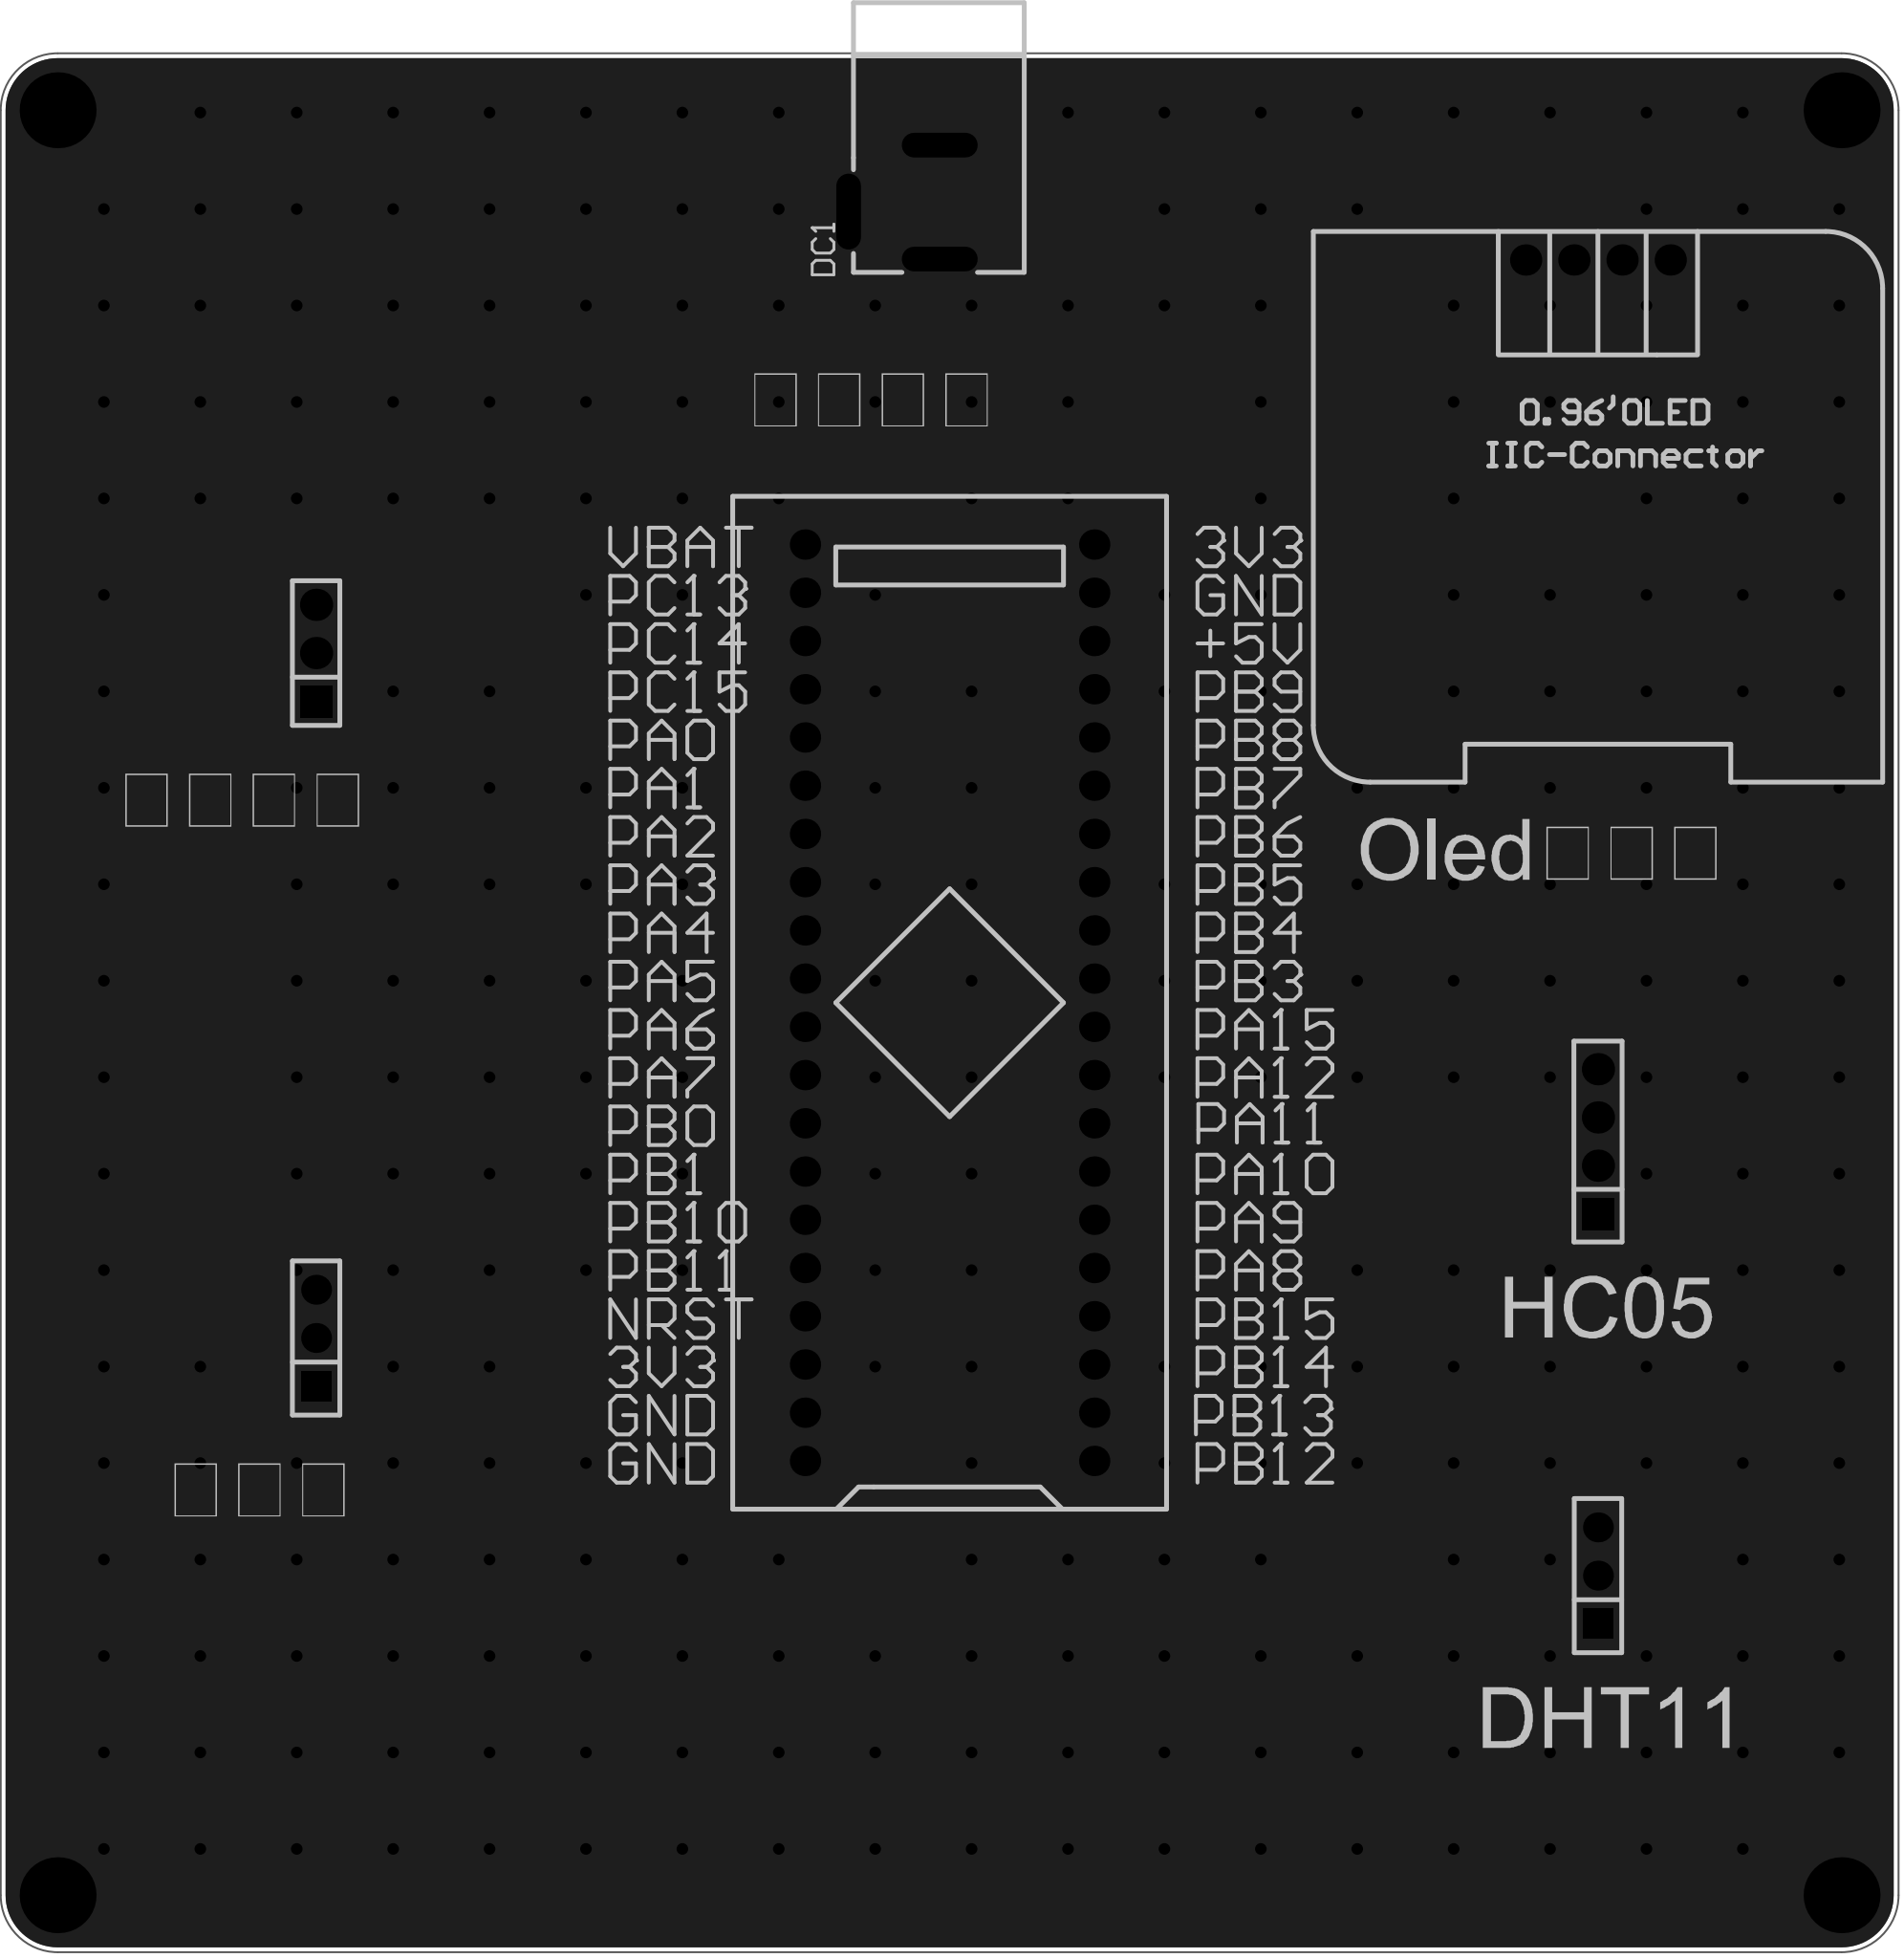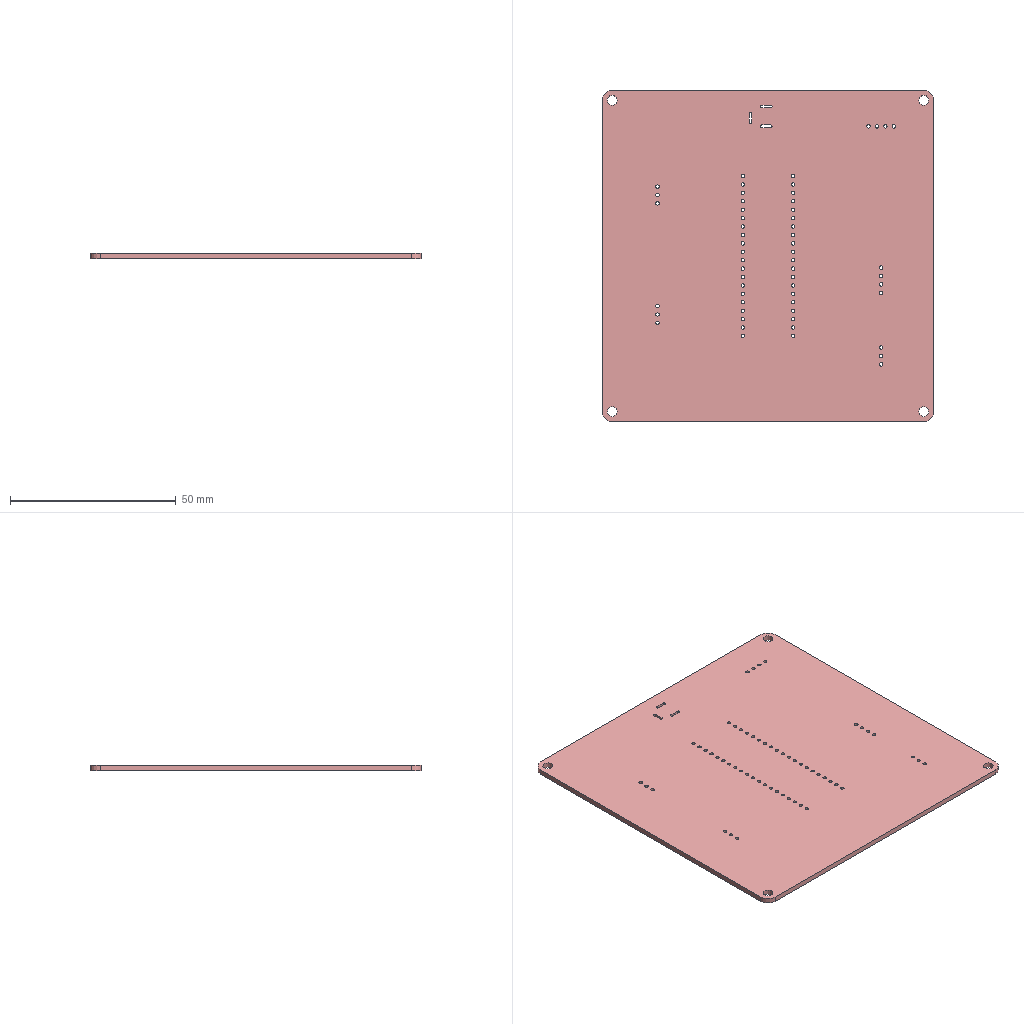Circuit board layout | Altium Designer | box 100 x 100 x 1.6 mm
Layer stack:
# Altium Designer layer stack of  (unit mm; dielectric type: 0 none, 1 core, 2 prepreg, 3 surface material)
index,name,kind,layer,copper_thickness_mm,dielectric_type,dielectric_thickness_mm,dielectric_material,dielectric_constant
0,Top Paste Mask Layer,other,,,,,,
1,Top Silkscreen Layer,other,,,,,,
2,Top Solder Mask Layer,dielectric,,,3,0.01,,3.3
3,Top Layer,copper,Top Layer,0.035,,,,
4,Dielectric1,dielectric,,,3,1.51,FR4,4.5
5,Bottom Layer,copper,Bottom Layer,0.035,,,,
6,Bottom Solder Mask Layer,dielectric,,,3,0.01,,3.3
7,Bottom Silkscreen Layer,other,,,,,,
8,Bottom Paste Mask Layer,other,,,,,,
# drill layer pairs: low layer,high layer
drill_pair,Top Layer,Bottom Layer
Part placement:
Designator,Comment,Layer,Footprint,Center-X(mm),Center-Y(mm),Rotation
U1,STM32F103C8T6-Card,TopLayer,CONN-TH_L53.3-W22.9_STM32F103C8T6-CARD,141.351,130.937,90
OLED1,,TopLayer,0.96OLED_4P,175.514,170.053,0
H1,,TopLayer,HDR-TH_3P-P2.54-V-F,107.97,113.282,90
H2,,TopLayer,HDR-TH_4P-P2.54-V-F,175.514,123.626,90
H3,,TopLayer,HDR-TH_3P-P2.54-V-F,175.514,100.768,90
H4,,TopLayer,HDR-TH_3P-P2.54-V-M,107.97,149.352,90
DC1,,TopLayer,DC-2.0,138.43,173.101,90
Pad and via stacks:
# Altium Designer via and pad stacks of  (unit mm). Each distinct definition once, with the count of objects using it.
# via: kind,start_layer,end_layer,hole_mm,diameter_mm,mode(0 simple;1 top-mid-bottom;2 full stack),diameter_per_layer,count,example_net
# pad: kind,layer,hole_mm,hole_type(0 round;1 square;2 slot),plating,top_size,top_shape(1 round;2 rect;3 octagon;9 rounded rect),mid_size,bottom_size,mode,footprint,size_per_layer,count,example
pad,Multi-Layer,3,0,plated,4x4,1,4x4,4x4,0,,,4,1
pad,Multi-Layer,1,0,plated,1.6x1.6,1,1.6x1.6,1.6x1.6,0,CONN-TH_L53.3-W22.9_STM32F103C8T6-CARD,,40,U1.1
pad,Multi-Layer,1,0,plated,1.65x1.65,1,1.65x1.65,1.65x1.65,0,0.96OLED_4P,,4,OLED1.4
pad,Multi-Layer,1.02,0,plated,1.575x1.575,1,1.575x1.575,1.575x1.575,0,HDR-TH_3P-P2.54-V-F,,4,H1.3
pad,Multi-Layer,1.02,0,plated,1.575x1.575,2,1.575x1.575,1.575x1.575,0,HDR-TH_3P-P2.54-V-F,,2,H1.1
pad,Multi-Layer,1.1,0,plated,1.7x1.7,2,1.7x1.7,1.7x1.7,0,HDR-TH_4P-P2.54-V-F,,1,H2.1
pad,Multi-Layer,1.1,0,plated,1.7x1.7,1,1.7x1.7,1.7x1.7,0,HDR-TH_4P-P2.54-V-F,,3,H2.2
pad,Multi-Layer,1.1,0,plated,1.7x1.7,2,1.7x1.7,1.7x1.7,0,HDR-TH_3P-P2.54-V-M,,1,H4.1
pad,Multi-Layer,1.1,0,plated,1.7x1.7,1,1.7x1.7,1.7x1.7,0,HDR-TH_3P-P2.54-V-M,,2,H4.2
pad,Multi-Layer,0.8001,2,plated,4x1.3,1,4x1.3,4x1.3,0,DC-2.0,,3,DC1.2
via,Top Layer,Bottom Layer,0.3048,0.61,0,,291,GND
Copper pours:
name,layer,net,type(0 solid;1 hatched;2 none)
Bottom Layer-GND,Bottom Layer,GND,0
Top Layer-GND,Top Layer,GND,0
Design rules, without the lines most boards share:
# Altium Designer design rules of  (exported by Altium Designer, unit mm)
# columns: name | kind | enabled | priority | scope1 | scope2 | descriptor | typed fields (field=value)
Copper_copperRegion_copperThickness1oz | 0 | disabled | 4 | All | All | Clearance Constraint (Gap=5.984mil) (Disabled)(All),(All) | gap=0.152
Copper_copperRegion_copperThickness1oz_1 | 63 | disabled | 4 | All | All | Board Clearance Constraint (Gap=0mil) (Disabled)(All) |
Copper_copperRegion_Copper_copperRegion | 0 | disabled | 5 | All | All | Clearance Constraint (Gap=5.984mil) (Disabled)(All),(All) | gap=0.152
Copper_copperRegion_Copper_copperRegion_1 | 63 | disabled | 5 | All | All | Board Clearance Constraint (Gap=0mil) (Disabled)(All) |
copperThickness1oz | 0 | enabled | 6 | All | All | Clearance Constraint (Gap=5.984mil) (All),(All) | gap=0.152
copperThickness1oz_1 | 63 | enabled | 6 | All | All | Board Clearance Constraint (Gap=0mil) (All) |
copperRegion_copperThickness1oz | 20 | disabled | 1 | All | All | Polygon Connect Rule(Relief Connect )(Conductor Width=10mil) (Relief Angle=90 Angle) (Entries=4) (Air Gap Width=10mil) (Disabled)(All),(All) | connect_style(0=relief,1=direct,2=none)=0 relief_conductor_width=0.254 relief_entries=4
copperRegion_Copper_copperRegion | 20 | disabled | 2 | All | All | Polygon Connect Rule(Relief Connect )(Conductor Width=10mil) (Relief Angle=90 Angle) (Entries=4) (Air Gap Width=10mil) (Disabled)(All),(All) | connect_style(0=relief,1=direct,2=none)=0 relief_conductor_width=0.254 relief_entries=4
copperRegion | 20 | enabled | 3 | All | All | Polygon Connect Rule(Relief Connect )(Conductor Width=10mil) (Relief Angle=90 Angle) (Entries=4) (Air Gap Width=10mil) (All),(All) | connect_style(0=relief,1=direct,2=none)=0 relief_conductor_width=0.254 relief_entries=4